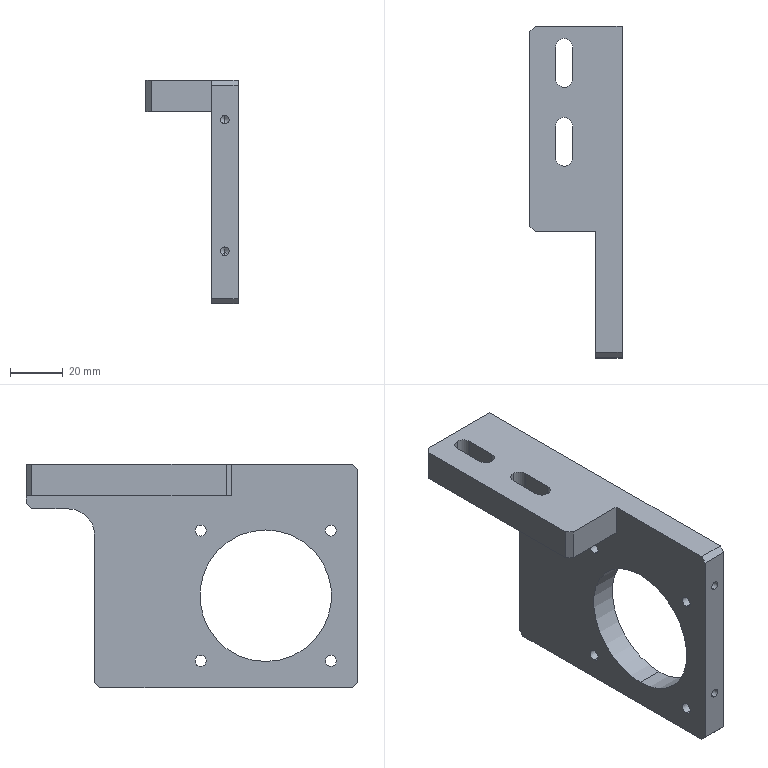Part | SolidWorks | features BaseBody 1 | 1 solid | 54 faces | box 35 x 126 x 85 mm | volume 89570 mm3 | cylinder 25 | plane 21 | cone 8 | commonest cylinder face diameters 3.3 x8 4.2 x8 6.6 x6 50 x2 20 x1